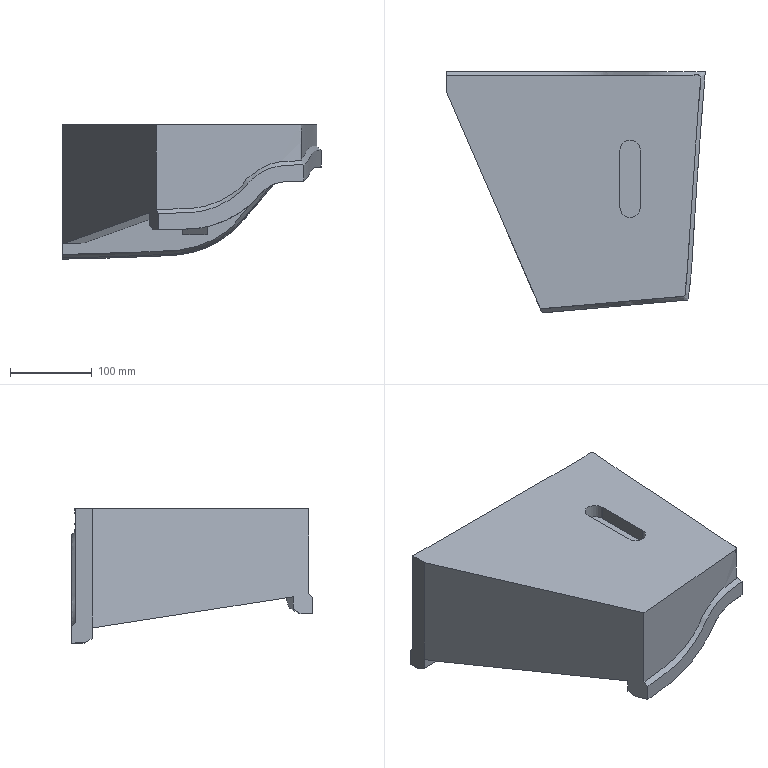Part | NX | features solid 2 | 1 solid | 53 faces | box 318.135 x 296.607 x 164.841 mm | volume 4477902 mm3 | plane 27 | spline 18 | cylinder 8 | commonest cylinder face diameters 30 x6 25 x2